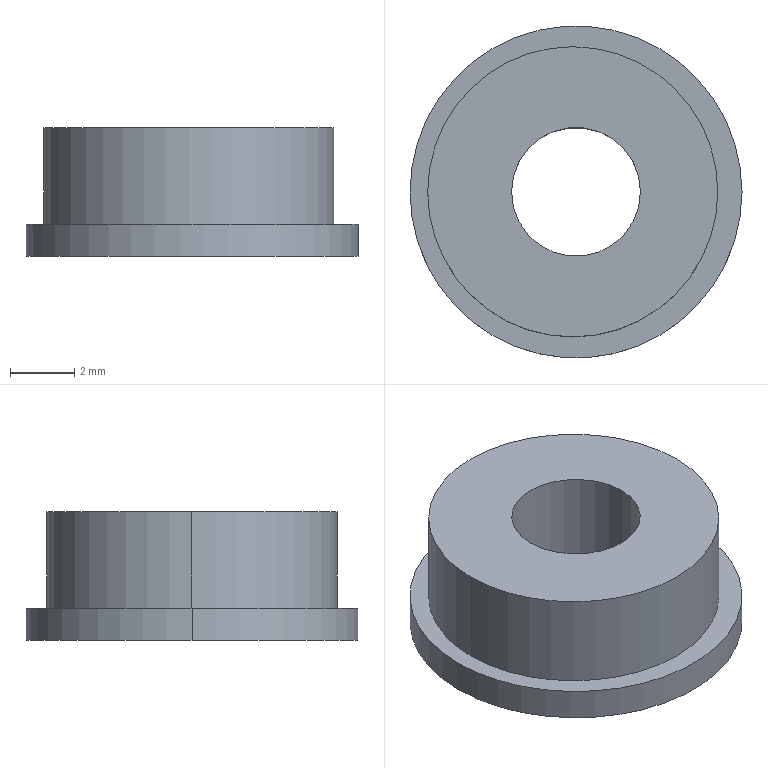Part | SolidWorks | features Extrusion 1, ICE 1 | 1 solid | 9 faces | box 10.3 x 10.3 x 4 mm | volume 223.909 mm3 | cylinder 6 | plane 3 | commonest cylinder face diameters 4 x2 9 x2 10.3 x2
STEP:
#1=CARTESIAN_POINT('',(4.399,0.,1.));
#2=VERTEX_POINT('',#1);
#3=CARTESIAN_POINT('',(-4.601,0.,1.));
#4=VERTEX_POINT('',#3);
#5=CARTESIAN_POINT('',(-0.1013,0.,1.));
#6=DIRECTION('',(0.,0.,1.));
#7=DIRECTION('',(1.,0.,0.));
#8=AXIS2_PLACEMENT_3D('',#5,#6,#7);
#9=CIRCLE('',#8,4.5);
#10=EDGE_CURVE('',#2,#4,#9,.T.);
#11=ORIENTED_EDGE('',*,*,#10,.T.);
#12=CARTESIAN_POINT('',(-4.601,0.,4.));
#13=VERTEX_POINT('',#12);
#14=CARTESIAN_POINT('',(-4.601,0.,1.));
#15=DIRECTION('',(0.,0.,1.));
#16=VECTOR('',#15,1000.);
#17=LINE('',#14,#16);
#18=EDGE_CURVE('',#4,#13,#17,.T.);
#19=ORIENTED_EDGE('',*,*,#18,.T.);
#20=CARTESIAN_POINT('',(4.399,0.,4.));
#21=VERTEX_POINT('',#20);
#22=CARTESIAN_POINT('',(-0.1013,0.,4.));
#23=DIRECTION('',(0.,0.,1.));
#24=DIRECTION('',(1.,0.,0.));
#25=AXIS2_PLACEMENT_3D('',#22,#23,#24);
#26=CIRCLE('',#25,4.5);
#27=EDGE_CURVE('',#21,#13,#26,.T.);
#28=ORIENTED_EDGE('',*,*,#27,.F.);
#29=CARTESIAN_POINT('',(4.399,0.,1.));
#30=DIRECTION('',(0.,0.,1.));
#31=VECTOR('',#30,1000.);
#32=LINE('',#29,#31);
#33=EDGE_CURVE('',#2,#21,#32,.T.);
#34=ORIENTED_EDGE('',*,*,#33,.F.);
#35=EDGE_LOOP('',(#11,#19,#28,#34));
#36=FACE_OUTER_BOUND('',#35,.T.);
#37=CARTESIAN_POINT('',(-0.1013,0.,1.));
#38=DIRECTION('',(0.,0.,1.));
#39=DIRECTION('',(1.,0.,0.));
#40=AXIS2_PLACEMENT_3D('',#37,#38,#39);
#41=CYLINDRICAL_SURFACE('',#40,4.5);
#42=ADVANCED_FACE('',(#36),#41,.T.);
#43=CARTESIAN_POINT('',(-2.,0.,4.));
#44=VERTEX_POINT('',#43);
#45=CARTESIAN_POINT('',(2.,0.,4.));
#46=VERTEX_POINT('',#45);
#47=CARTESIAN_POINT('',(0.,0.,4.));
#48=DIRECTION('',(0.,0.,1.));
#49=DIRECTION('',(1.,0.,0.));
#50=AXIS2_PLACEMENT_3D('',#47,#48,#49);
#51=CIRCLE('',#50,2.);
#52=EDGE_CURVE('',#44,#46,#51,.T.);
#53=ORIENTED_EDGE('',*,*,#52,.T.);
#54=CARTESIAN_POINT('',(2.,0.,0.));
#55=VERTEX_POINT('',#54);
#56=CARTESIAN_POINT('',(2.,0.,4.));
#57=DIRECTION('',(0.,0.,-1.));
#58=VECTOR('',#57,1000.);
#59=LINE('',#56,#58);
#60=EDGE_CURVE('',#46,#55,#59,.T.);
#61=ORIENTED_EDGE('',*,*,#60,.T.);
#62=CARTESIAN_POINT('',(-2.,0.,0.));
#63=VERTEX_POINT('',#62);
#64=CARTESIAN_POINT('',(0.,0.,0.));
#65=DIRECTION('',(0.,0.,1.));
#66=DIRECTION('',(1.,0.,0.));
#67=AXIS2_PLACEMENT_3D('',#64,#65,#66);
#68=CIRCLE('',#67,2.);
#69=EDGE_CURVE('',#63,#55,#68,.T.);
#70=ORIENTED_EDGE('',*,*,#69,.F.);
#71=CARTESIAN_POINT('',(-2.,0.,4.));
#72=DIRECTION('',(0.,0.,-1.));
#73=VECTOR('',#72,1000.);
#74=LINE('',#71,#73);
#75=EDGE_CURVE('',#44,#63,#74,.T.);
#76=ORIENTED_EDGE('',*,*,#75,.F.);
#77=EDGE_LOOP('',(#53,#61,#70,#76));
#78=FACE_OUTER_BOUND('',#77,.T.);
#79=CARTESIAN_POINT('',(0.,0.,4.));
#80=DIRECTION('',(0.,0.,-1.));
#81=DIRECTION('',(-1.,0.,0.));
#82=AXIS2_PLACEMENT_3D('',#79,#80,#81);
#83=CYLINDRICAL_SURFACE('',#82,2.);
#84=ADVANCED_FACE('',(#78),#83,.F.);
#85=CARTESIAN_POINT('',(5.15,0.,1.));
#86=VERTEX_POINT('',#85);
#87=CARTESIAN_POINT('',(-5.15,0.,1.));
#88=VERTEX_POINT('',#87);
#89=CARTESIAN_POINT('',(0.,0.,1.));
#90=DIRECTION('',(0.,0.,1.));
#91=DIRECTION('',(1.,0.,0.));
#92=AXIS2_PLACEMENT_3D('',#89,#90,#91);
#93=CIRCLE('',#92,5.15);
#94=EDGE_CURVE('',#86,#88,#93,.T.);
#95=ORIENTED_EDGE('',*,*,#94,.F.);
#96=CARTESIAN_POINT('',(5.15,0.,0.));
#97=VERTEX_POINT('',#96);
#98=CARTESIAN_POINT('',(5.15,0.,4.));
#99=DIRECTION('',(0.,0.,-1.));
#100=VECTOR('',#99,1000.);
#101=LINE('',#98,#100);
#102=EDGE_CURVE('',#86,#97,#101,.T.);
#103=ORIENTED_EDGE('',*,*,#102,.T.);
#104=CARTESIAN_POINT('',(-5.15,0.,0.));
#105=VERTEX_POINT('',#104);
#106=CARTESIAN_POINT('',(0.,0.,0.));
#107=DIRECTION('',(0.,0.,1.));
#108=DIRECTION('',(1.,0.,0.));
#109=AXIS2_PLACEMENT_3D('',#106,#107,#108);
#110=CIRCLE('',#109,5.15);
#111=EDGE_CURVE('',#97,#105,#110,.T.);
#112=ORIENTED_EDGE('',*,*,#111,.T.);
#113=CARTESIAN_POINT('',(-5.15,0.,4.));
#114=DIRECTION('',(0.,0.,-1.));
#115=VECTOR('',#114,1000.);
#116=LINE('',#113,#115);
#117=EDGE_CURVE('',#88,#105,#116,.T.);
#118=ORIENTED_EDGE('',*,*,#117,.F.);
#119=EDGE_LOOP('',(#95,#103,#112,#118));
#120=FACE_OUTER_BOUND('',#119,.T.);
#121=CARTESIAN_POINT('',(0.,0.,4.));
#122=DIRECTION('',(0.,0.,-1.));
#123=DIRECTION('',(-1.,0.,0.));
#124=AXIS2_PLACEMENT_3D('',#121,#122,#123);
#125=CYLINDRICAL_SURFACE('',#124,5.15);
#126=ADVANCED_FACE('',(#120),#125,.T.);
#127=ORIENTED_EDGE('',*,*,#52,.F.);
#128=CARTESIAN_POINT('',(0.,0.,4.));
#129=DIRECTION('',(0.,0.,1.));
#130=DIRECTION('',(1.,0.,0.));
#131=AXIS2_PLACEMENT_3D('',#128,#129,#130);
#132=CIRCLE('',#131,2.);
#133=EDGE_CURVE('',#46,#44,#132,.T.);
#134=ORIENTED_EDGE('',*,*,#133,.F.);
#135=EDGE_LOOP('',(#127,#134));
#136=FACE_BOUND('',#135,.T.);
#137=ORIENTED_EDGE('',*,*,#27,.T.);
#138=CARTESIAN_POINT('',(-0.1013,0.,4.));
#139=DIRECTION('',(0.,0.,1.));
#140=DIRECTION('',(1.,0.,0.));
#141=AXIS2_PLACEMENT_3D('',#138,#139,#140);
#142=CIRCLE('',#141,4.5);
#143=EDGE_CURVE('',#13,#21,#142,.T.);
#144=ORIENTED_EDGE('',*,*,#143,.T.);
#145=EDGE_LOOP('',(#137,#144));
#146=FACE_OUTER_BOUND('',#145,.T.);
#147=CARTESIAN_POINT('',(0.,0.,4.));
#148=DIRECTION('',(0.,0.,1.));
#149=DIRECTION('',(1.,0.,0.));
#150=AXIS2_PLACEMENT_3D('',#147,#148,#149);
#151=PLANE('',#150);
#152=ADVANCED_FACE('',(#136,#146),#151,.T.);
#153=ORIENTED_EDGE('',*,*,#102,.F.);
#154=CARTESIAN_POINT('',(0.,0.,1.));
#155=DIRECTION('',(0.,0.,1.));
#156=DIRECTION('',(1.,0.,0.));
#157=AXIS2_PLACEMENT_3D('',#154,#155,#156);
#158=CIRCLE('',#157,5.15);
#159=EDGE_CURVE('',#88,#86,#158,.T.);
#160=ORIENTED_EDGE('',*,*,#159,.F.);
#161=ORIENTED_EDGE('',*,*,#117,.T.);
#162=CARTESIAN_POINT('',(0.,0.,0.));
#163=DIRECTION('',(0.,0.,1.));
#164=DIRECTION('',(1.,0.,0.));
#165=AXIS2_PLACEMENT_3D('',#162,#163,#164);
#166=CIRCLE('',#165,5.15);
#167=EDGE_CURVE('',#105,#97,#166,.T.);
#168=ORIENTED_EDGE('',*,*,#167,.T.);
#169=EDGE_LOOP('',(#153,#160,#161,#168));
#170=FACE_OUTER_BOUND('',#169,.T.);
#171=CARTESIAN_POINT('',(0.,0.,4.));
#172=DIRECTION('',(0.,0.,-1.));
#173=DIRECTION('',(-1.,0.,0.));
#174=AXIS2_PLACEMENT_3D('',#171,#172,#173);
#175=CYLINDRICAL_SURFACE('',#174,5.15);
#176=ADVANCED_FACE('',(#170),#175,.T.);
#177=ORIENTED_EDGE('',*,*,#167,.F.);
#178=ORIENTED_EDGE('',*,*,#111,.F.);
#179=EDGE_LOOP('',(#177,#178));
#180=FACE_OUTER_BOUND('',#179,.T.);
#181=ORIENTED_EDGE('',*,*,#69,.T.);
#182=CARTESIAN_POINT('',(0.,0.,0.));
#183=DIRECTION('',(0.,0.,1.));
#184=DIRECTION('',(1.,0.,0.));
#185=AXIS2_PLACEMENT_3D('',#182,#183,#184);
#186=CIRCLE('',#185,2.);
#187=EDGE_CURVE('',#55,#63,#186,.T.);
#188=ORIENTED_EDGE('',*,*,#187,.T.);
#189=EDGE_LOOP('',(#181,#188));
#190=FACE_BOUND('',#189,.T.);
#191=CARTESIAN_POINT('',(0.,0.,0.));
#192=DIRECTION('',(0.,0.,1.));
#193=DIRECTION('',(1.,0.,0.));
#194=AXIS2_PLACEMENT_3D('',#191,#192,#193);
#195=PLANE('',#194);
#196=ADVANCED_FACE('',(#180,#190),#195,.F.);
#197=ORIENTED_EDGE('',*,*,#60,.F.);
#198=ORIENTED_EDGE('',*,*,#133,.T.);
#199=ORIENTED_EDGE('',*,*,#75,.T.);
#200=ORIENTED_EDGE('',*,*,#187,.F.);
#201=EDGE_LOOP('',(#197,#198,#199,#200));
#202=FACE_OUTER_BOUND('',#201,.T.);
#203=CARTESIAN_POINT('',(0.,0.,4.));
#204=DIRECTION('',(0.,0.,-1.));
#205=DIRECTION('',(-1.,0.,0.));
#206=AXIS2_PLACEMENT_3D('',#203,#204,#205);
#207=CYLINDRICAL_SURFACE('',#206,2.);
#208=ADVANCED_FACE('',(#202),#207,.F.);
#209=ORIENTED_EDGE('',*,*,#10,.F.);
#210=CARTESIAN_POINT('',(-0.1013,0.,1.));
#211=DIRECTION('',(0.,0.,1.));
#212=DIRECTION('',(1.,0.,0.));
#213=AXIS2_PLACEMENT_3D('',#210,#211,#212);
#214=CIRCLE('',#213,4.5);
#215=EDGE_CURVE('',#4,#2,#214,.T.);
#216=ORIENTED_EDGE('',*,*,#215,.F.);
#217=EDGE_LOOP('',(#209,#216));
#218=FACE_BOUND('',#217,.T.);
#219=ORIENTED_EDGE('',*,*,#159,.T.);
#220=ORIENTED_EDGE('',*,*,#94,.T.);
#221=EDGE_LOOP('',(#219,#220));
#222=FACE_OUTER_BOUND('',#221,.T.);
#223=CARTESIAN_POINT('',(0.,0.,1.));
#224=DIRECTION('',(0.,0.,1.));
#225=DIRECTION('',(1.,0.,0.));
#226=AXIS2_PLACEMENT_3D('',#223,#224,#225);
#227=PLANE('',#226);
#228=ADVANCED_FACE('',(#218,#222),#227,.T.);
#229=ORIENTED_EDGE('',*,*,#18,.F.);
#230=ORIENTED_EDGE('',*,*,#215,.T.);
#231=ORIENTED_EDGE('',*,*,#33,.T.);
#232=ORIENTED_EDGE('',*,*,#143,.F.);
#233=EDGE_LOOP('',(#229,#230,#231,#232));
#234=FACE_OUTER_BOUND('',#233,.T.);
#235=CARTESIAN_POINT('',(-0.1013,0.,1.));
#236=DIRECTION('',(0.,0.,1.));
#237=DIRECTION('',(1.,0.,0.));
#238=AXIS2_PLACEMENT_3D('',#235,#236,#237);
#239=CYLINDRICAL_SURFACE('',#238,4.5);
#240=ADVANCED_FACE('',(#234),#239,.T.);
#241=CLOSED_SHELL('',(#42,#84,#126,#152,#176,#196,#208,#228,#240));
#242=MANIFOLD_SOLID_BREP('',#241);
#243=CARTESIAN_POINT('',(0.,0.,0.));
#244=DIRECTION('',(0.,0.,1.));
#245=DIRECTION('',(1.,0.,0.));
#246=AXIS2_PLACEMENT_3D('',#243,#244,#245);
#247=(LENGTH_UNIT()NAMED_UNIT(*)SI_UNIT(.MILLI.,.METRE.));
#248=UNCERTAINTY_MEASURE_WITH_UNIT(LENGTH_MEASURE(0.00001),#247,'','');
#249=(NAMED_UNIT(*)PLANE_ANGLE_UNIT()SI_UNIT($,.RADIAN.));
#250=(NAMED_UNIT(*)SI_UNIT($,.STERADIAN.)SOLID_ANGLE_UNIT());
#251=(GEOMETRIC_REPRESENTATION_CONTEXT(3)GLOBAL_UNCERTAINTY_ASSIGNED_CONTEXT((#248))GLOBAL_UNIT_ASSIGNED_CONTEXT((#247,#249,#250))REPRESENTATION_CONTEXT('',''));
#252=ADVANCED_BREP_SHAPE_REPRESENTATION('',(#242,#246),#251);